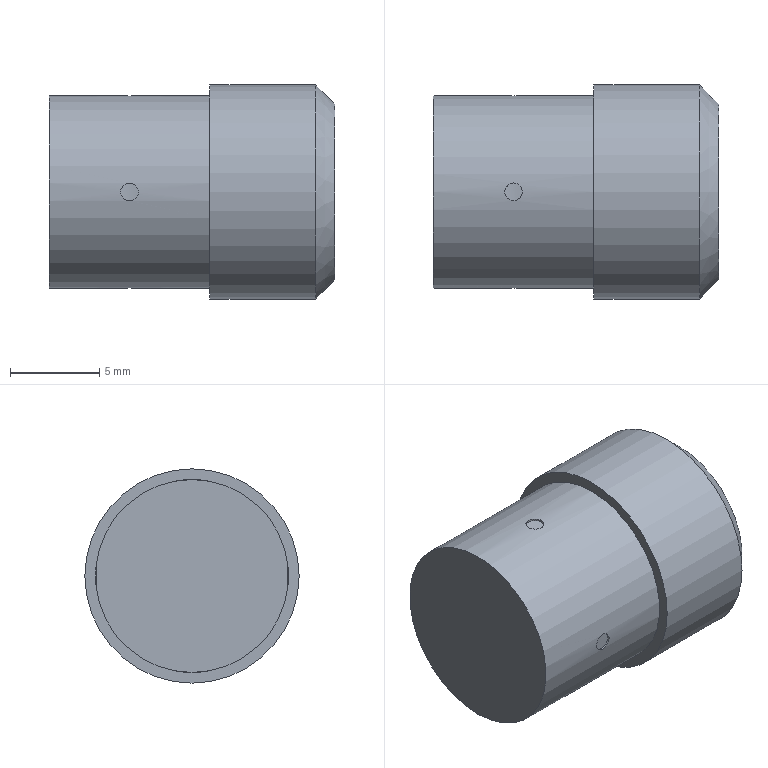Part | NX | features BREP 1 | 1 solid | 24 faces | box 16 x 12 x 12 mm | volume 1208 mm3 | cylinder 15 | plane 8 | cone 1 | commonest cylinder face diameters 1 x8 10.6 x4 9.6 x1 10.8 x1 12 x1
STEP:
#1=CARTESIAN_POINT('',(4.,0.,5.4));
#2=VERTEX_POINT('',#1);
#3=CARTESIAN_POINT('',(4.501,-0.7501,5.354));
#4=CARTESIAN_POINT('',(3.75,0.00004561,5.423));
#5=CARTESIAN_POINT('',(4.5,0.7499,5.354));
#6=CARTESIAN_POINT('',(5.25,0.0003197,5.423));
#7=CARTESIAN_POINT('',(4.501,-0.7501,5.354));
#8=CARTESIAN_POINT('',(3.75,0.00004561,5.423));
#9=CARTESIAN_POINT('',(4.5,0.7499,5.354));
#10=B_SPLINE_CURVE_WITH_KNOTS('',3,(#3,#4,#5,#6,#7,#8,#9),.UNSPECIFIED.,.T.,.F.,(1,1,1,1,1,1,1,1,1,1,1),(-0.002346,-0.001564,-0.0007819,0.,0.0007819,0.001564,0.002346,0.003128,0.00391,0.004692,0.005474),.UNSPECIFIED.);
#11=EDGE_CURVE('',#2,#2,#10,.T.);
#12=ORIENTED_EDGE('',*,*,#11,.T.);
#13=EDGE_LOOP('',(#12));
#14=FACE_BOUND('',#13,.T.);
#15=CARTESIAN_POINT('',(9.,0.,-5.4));
#16=VERTEX_POINT('',#15);
#17=CARTESIAN_POINT('',(9.,0.,0.));
#18=DIRECTION('',(-1.,0.,0.));
#19=DIRECTION('',(0.,0.,-1.));
#20=AXIS2_PLACEMENT_3D('',#17,#18,#19);
#21=CIRCLE('',#20,5.4);
#22=EDGE_CURVE('',#16,#16,#21,.T.);
#23=ORIENTED_EDGE('',*,*,#22,.T.);
#24=EDGE_LOOP('',(#23));
#25=FACE_BOUND('',#24,.T.);
#26=CARTESIAN_POINT('',(5.,0.,-5.4));
#27=VERTEX_POINT('',#26);
#28=CARTESIAN_POINT('',(4.499,-0.7501,-5.354));
#29=CARTESIAN_POINT('',(5.25,0.00004561,-5.423));
#30=CARTESIAN_POINT('',(4.5,0.7499,-5.354));
#31=CARTESIAN_POINT('',(3.75,0.0003197,-5.423));
#32=CARTESIAN_POINT('',(4.499,-0.7501,-5.354));
#33=CARTESIAN_POINT('',(5.25,0.00004561,-5.423));
#34=CARTESIAN_POINT('',(4.5,0.7499,-5.354));
#35=B_SPLINE_CURVE_WITH_KNOTS('',3,(#28,#29,#30,#31,#32,#33,#34),.UNSPECIFIED.,.T.,.F.,(1,1,1,1,1,1,1,1,1,1,1),(-0.002346,-0.001564,-0.0007819,0.,0.0007819,0.001564,0.002346,0.003128,0.00391,0.004692,0.005474),.UNSPECIFIED.);
#36=EDGE_CURVE('',#27,#27,#35,.T.);
#37=ORIENTED_EDGE('',*,*,#36,.T.);
#38=EDGE_LOOP('',(#37));
#39=FACE_BOUND('',#38,.T.);
#40=CARTESIAN_POINT('',(0.,0.,-5.4));
#41=VERTEX_POINT('',#40);
#42=CARTESIAN_POINT('',(0.,0.,0.));
#43=DIRECTION('',(1.,0.,0.));
#44=DIRECTION('',(0.,0.,-1.));
#45=AXIS2_PLACEMENT_3D('',#42,#43,#44);
#46=CIRCLE('',#45,5.4);
#47=EDGE_CURVE('',#41,#41,#46,.T.);
#48=ORIENTED_EDGE('',*,*,#47,.T.);
#49=EDGE_LOOP('',(#48));
#50=FACE_BOUND('',#49,.T.);
#51=CARTESIAN_POINT('',(4.5,5.377,0.5));
#52=VERTEX_POINT('',#51);
#53=CARTESIAN_POINT('',(5.25,5.423,-0.0007741));
#54=CARTESIAN_POINT('',(4.5,5.354,0.7501));
#55=CARTESIAN_POINT('',(3.75,5.423,0.0003559));
#56=CARTESIAN_POINT('',(4.5,5.354,-0.7499));
#57=CARTESIAN_POINT('',(5.25,5.423,-0.0007741));
#58=CARTESIAN_POINT('',(4.5,5.354,0.7501));
#59=CARTESIAN_POINT('',(3.75,5.423,0.0003559));
#60=B_SPLINE_CURVE_WITH_KNOTS('',3,(#53,#54,#55,#56,#57,#58,#59),.UNSPECIFIED.,.T.,.F.,(1,1,1,1,1,1,1,1,1,1,1),(-0.002346,-0.001564,-0.0007819,0.,0.0007819,0.001564,0.002346,0.003128,0.00391,0.004692,0.005474),.UNSPECIFIED.);
#61=EDGE_CURVE('',#52,#52,#60,.T.);
#62=ORIENTED_EDGE('',*,*,#61,.T.);
#63=EDGE_LOOP('',(#62));
#64=FACE_BOUND('',#63,.T.);
#65=CARTESIAN_POINT('',(4.5,-5.377,-0.5));
#66=VERTEX_POINT('',#65);
#67=CARTESIAN_POINT('',(5.25,-5.423,0.0007741));
#68=CARTESIAN_POINT('',(4.5,-5.354,-0.7501));
#69=CARTESIAN_POINT('',(3.75,-5.423,-0.0003559));
#70=CARTESIAN_POINT('',(4.5,-5.354,0.7499));
#71=CARTESIAN_POINT('',(5.25,-5.423,0.0007741));
#72=CARTESIAN_POINT('',(4.5,-5.354,-0.7501));
#73=CARTESIAN_POINT('',(3.75,-5.423,-0.0003559));
#74=B_SPLINE_CURVE_WITH_KNOTS('',3,(#67,#68,#69,#70,#71,#72,#73),.UNSPECIFIED.,.T.,.F.,(1,1,1,1,1,1,1,1,1,1,1),(-0.002346,-0.001564,-0.0007819,0.,0.0007819,0.001564,0.002346,0.003128,0.00391,0.004692,0.005474),.UNSPECIFIED.);
#75=EDGE_CURVE('',#66,#66,#74,.T.);
#76=ORIENTED_EDGE('',*,*,#75,.T.);
#77=EDGE_LOOP('',(#76));
#78=FACE_BOUND('',#77,.T.);
#79=CARTESIAN_POINT('',(9.,0.,0.));
#80=DIRECTION('',(1.,0.,0.));
#81=DIRECTION('',(0.,0.,1.));
#82=AXIS2_PLACEMENT_3D('',#79,#80,#81);
#83=CYLINDRICAL_SURFACE('',#82,5.4);
#84=ADVANCED_FACE('',(#14,#25,#39,#50,#64,#78),#83,.T.);
#85=ORIENTED_EDGE('',*,*,#36,.F.);
#86=EDGE_LOOP('',(#85));
#87=FACE_BOUND('',#86,.T.);
#88=CARTESIAN_POINT('',(4.,0.,-5.3));
#89=VERTEX_POINT('',#88);
#90=CARTESIAN_POINT('',(4.501,-0.7501,-5.253));
#91=CARTESIAN_POINT('',(3.75,0.00004567,-5.324));
#92=CARTESIAN_POINT('',(4.5,0.7499,-5.253));
#93=CARTESIAN_POINT('',(5.25,0.0003201,-5.324));
#94=CARTESIAN_POINT('',(4.501,-0.7501,-5.253));
#95=CARTESIAN_POINT('',(3.75,0.00004567,-5.324));
#96=CARTESIAN_POINT('',(4.5,0.7499,-5.253));
#97=B_SPLINE_CURVE_WITH_KNOTS('',3,(#90,#91,#92,#93,#94,#95,#96),.UNSPECIFIED.,.T.,.F.,(1,1,1,1,1,1,1,1,1,1,1),(-0.002346,-0.001564,-0.000782,0.,0.000782,0.001564,0.002346,0.003128,0.00391,0.004692,0.005474),.UNSPECIFIED.);
#98=EDGE_CURVE('',#89,#89,#97,.T.);
#99=ORIENTED_EDGE('',*,*,#98,.F.);
#100=EDGE_LOOP('',(#99));
#101=FACE_BOUND('',#100,.T.);
#102=CARTESIAN_POINT('',(4.5,0.,0.));
#103=DIRECTION('',(0.,0.,1.));
#104=DIRECTION('',(-1.,0.,0.));
#105=AXIS2_PLACEMENT_3D('',#102,#103,#104);
#106=CYLINDRICAL_SURFACE('',#105,0.5);
#107=ADVANCED_FACE('',(#87,#101),#106,.F.);
#108=ORIENTED_EDGE('',*,*,#22,.F.);
#109=EDGE_LOOP('',(#108));
#110=FACE_BOUND('',#109,.T.);
#111=CARTESIAN_POINT('',(9.,0.,-6.));
#112=VERTEX_POINT('',#111);
#113=CARTESIAN_POINT('',(9.,0.,0.));
#114=DIRECTION('',(1.,0.,0.));
#115=DIRECTION('',(0.,0.,-1.));
#116=AXIS2_PLACEMENT_3D('',#113,#114,#115);
#117=CIRCLE('',#116,6.);
#118=EDGE_CURVE('',#112,#112,#117,.T.);
#119=ORIENTED_EDGE('',*,*,#118,.F.);
#120=EDGE_LOOP('',(#119));
#121=FACE_BOUND('',#120,.T.);
#122=CARTESIAN_POINT('',(9.,0.,0.));
#123=DIRECTION('',(1.,0.,0.));
#124=DIRECTION('',(0.,0.,1.));
#125=AXIS2_PLACEMENT_3D('',#122,#123,#124);
#126=PLANE('',#125);
#127=ADVANCED_FACE('',(#110,#121),#126,.F.);
#128=CARTESIAN_POINT('',(5.,0.,5.3));
#129=VERTEX_POINT('',#128);
#130=CARTESIAN_POINT('',(4.499,-0.7501,5.253));
#131=CARTESIAN_POINT('',(5.25,0.00004567,5.324));
#132=CARTESIAN_POINT('',(4.5,0.7499,5.253));
#133=CARTESIAN_POINT('',(3.75,0.0003201,5.324));
#134=CARTESIAN_POINT('',(4.499,-0.7501,5.253));
#135=CARTESIAN_POINT('',(5.25,0.00004567,5.324));
#136=CARTESIAN_POINT('',(4.5,0.7499,5.253));
#137=B_SPLINE_CURVE_WITH_KNOTS('',3,(#130,#131,#132,#133,#134,#135,#136),.UNSPECIFIED.,.T.,.F.,(1,1,1,1,1,1,1,1,1,1,1),(-0.002346,-0.001564,-0.000782,0.,0.000782,0.001564,0.002346,0.003128,0.00391,0.004692,0.005474),.UNSPECIFIED.);
#138=EDGE_CURVE('',#129,#129,#137,.T.);
#139=ORIENTED_EDGE('',*,*,#138,.F.);
#140=EDGE_LOOP('',(#139));
#141=FACE_BOUND('',#140,.T.);
#142=ORIENTED_EDGE('',*,*,#11,.F.);
#143=EDGE_LOOP('',(#142));
#144=FACE_BOUND('',#143,.T.);
#145=CARTESIAN_POINT('',(4.5,0.,5.4));
#146=DIRECTION('',(0.,0.,1.));
#147=DIRECTION('',(-1.,0.,0.));
#148=AXIS2_PLACEMENT_3D('',#145,#146,#147);
#149=CYLINDRICAL_SURFACE('',#148,0.5);
#150=ADVANCED_FACE('',(#141,#144),#149,.F.);
#151=ORIENTED_EDGE('',*,*,#47,.F.);
#152=EDGE_LOOP('',(#151));
#153=FACE_BOUND('',#152,.T.);
#154=CARTESIAN_POINT('',(0.,0.,0.));
#155=DIRECTION('',(1.,0.,0.));
#156=DIRECTION('',(0.,0.,1.));
#157=AXIS2_PLACEMENT_3D('',#154,#155,#156);
#158=PLANE('',#157);
#159=ADVANCED_FACE('',(#153),#158,.F.);
#160=ORIENTED_EDGE('',*,*,#61,.F.);
#161=EDGE_LOOP('',(#160));
#162=FACE_BOUND('',#161,.T.);
#163=CARTESIAN_POINT('',(4.5,5.276,0.5));
#164=VERTEX_POINT('',#163);
#165=CARTESIAN_POINT('',(3.75,5.324,-0.0007718));
#166=CARTESIAN_POINT('',(4.5,5.253,0.7501));
#167=CARTESIAN_POINT('',(5.25,5.324,0.0003567));
#168=CARTESIAN_POINT('',(4.5,5.253,-0.7499));
#169=CARTESIAN_POINT('',(3.75,5.324,-0.0007718));
#170=CARTESIAN_POINT('',(4.5,5.253,0.7501));
#171=CARTESIAN_POINT('',(5.25,5.324,0.0003567));
#172=B_SPLINE_CURVE_WITH_KNOTS('',3,(#165,#166,#167,#168,#169,#170,#171),.UNSPECIFIED.,.T.,.F.,(1,1,1,1,1,1,1,1,1,1,1),(-0.002346,-0.001564,-0.000782,0.,0.000782,0.001564,0.002346,0.003128,0.00391,0.004692,0.005474),.UNSPECIFIED.);
#173=EDGE_CURVE('',#164,#164,#172,.T.);
#174=ORIENTED_EDGE('',*,*,#173,.F.);
#175=EDGE_LOOP('',(#174));
#176=FACE_BOUND('',#175,.T.);
#177=CARTESIAN_POINT('',(4.5,0.,0.));
#178=DIRECTION('',(0.,-1.,0.));
#179=DIRECTION('',(0.,0.,1.));
#180=AXIS2_PLACEMENT_3D('',#177,#178,#179);
#181=CYLINDRICAL_SURFACE('',#180,0.5);
#182=ADVANCED_FACE('',(#162,#176),#181,.F.);
#183=ORIENTED_EDGE('',*,*,#75,.F.);
#184=EDGE_LOOP('',(#183));
#185=FACE_BOUND('',#184,.T.);
#186=CARTESIAN_POINT('',(4.5,-5.276,0.5));
#187=VERTEX_POINT('',#186);
#188=CARTESIAN_POINT('',(5.25,-5.324,-0.0007718));
#189=CARTESIAN_POINT('',(4.5,-5.253,0.7501));
#190=CARTESIAN_POINT('',(3.75,-5.324,0.0003567));
#191=CARTESIAN_POINT('',(4.5,-5.253,-0.7499));
#192=CARTESIAN_POINT('',(5.25,-5.324,-0.0007718));
#193=CARTESIAN_POINT('',(4.5,-5.253,0.7501));
#194=CARTESIAN_POINT('',(3.75,-5.324,0.0003567));
#195=B_SPLINE_CURVE_WITH_KNOTS('',3,(#188,#189,#190,#191,#192,#193,#194),.UNSPECIFIED.,.T.,.F.,(1,1,1,1,1,1,1,1,1,1,1),(-0.002346,-0.001564,-0.000782,0.,0.000782,0.001564,0.002346,0.003128,0.00391,0.004692,0.005474),.UNSPECIFIED.);
#196=EDGE_CURVE('',#187,#187,#195,.T.);
#197=ORIENTED_EDGE('',*,*,#196,.F.);
#198=EDGE_LOOP('',(#197));
#199=FACE_BOUND('',#198,.T.);
#200=CARTESIAN_POINT('',(4.5,0.,0.));
#201=DIRECTION('',(0.,-1.,0.));
#202=DIRECTION('',(0.,0.,1.));
#203=AXIS2_PLACEMENT_3D('',#200,#201,#202);
#204=CYLINDRICAL_SURFACE('',#203,0.5);
#205=ADVANCED_FACE('',(#185,#199),#204,.F.);
#206=ORIENTED_EDGE('',*,*,#98,.T.);
#207=EDGE_LOOP('',(#206));
#208=FACE_BOUND('',#207,.T.);
#209=CARTESIAN_POINT('',(9.,0.,0.));
#210=DIRECTION('',(1.,0.,0.));
#211=DIRECTION('',(0.,0.,1.));
#212=AXIS2_PLACEMENT_3D('',#209,#210,#211);
#213=CYLINDRICAL_SURFACE('',#212,5.3);
#214=ADVANCED_FACE('',(#208),#213,.T.);
#215=CARTESIAN_POINT('',(14.927,0.,-6.));
#216=VERTEX_POINT('',#215);
#217=CARTESIAN_POINT('',(14.927,0.,0.));
#218=DIRECTION('',(-1.,0.,0.));
#219=DIRECTION('',(0.,0.,-1.));
#220=AXIS2_PLACEMENT_3D('',#217,#218,#219);
#221=CIRCLE('',#220,6.);
#222=EDGE_CURVE('',#216,#216,#221,.T.);
#223=ORIENTED_EDGE('',*,*,#222,.T.);
#224=EDGE_LOOP('',(#223));
#225=FACE_BOUND('',#224,.T.);
#226=ORIENTED_EDGE('',*,*,#118,.T.);
#227=EDGE_LOOP('',(#226));
#228=FACE_BOUND('',#227,.T.);
#229=CARTESIAN_POINT('',(16.,0.,0.));
#230=DIRECTION('',(1.,0.,0.));
#231=DIRECTION('',(0.,0.,1.));
#232=AXIS2_PLACEMENT_3D('',#229,#230,#231);
#233=CYLINDRICAL_SURFACE('',#232,6.);
#234=ADVANCED_FACE('',(#225,#228),#233,.T.);
#235=ORIENTED_EDGE('',*,*,#138,.T.);
#236=EDGE_LOOP('',(#235));
#237=FACE_BOUND('',#236,.T.);
#238=CARTESIAN_POINT('',(9.,0.,0.));
#239=DIRECTION('',(1.,0.,0.));
#240=DIRECTION('',(0.,0.,1.));
#241=AXIS2_PLACEMENT_3D('',#238,#239,#240);
#242=CYLINDRICAL_SURFACE('',#241,5.3);
#243=ADVANCED_FACE('',(#237),#242,.T.);
#244=ORIENTED_EDGE('',*,*,#173,.T.);
#245=EDGE_LOOP('',(#244));
#246=FACE_BOUND('',#245,.T.);
#247=CARTESIAN_POINT('',(9.,0.,0.));
#248=DIRECTION('',(1.,0.,0.));
#249=DIRECTION('',(0.,0.,1.));
#250=AXIS2_PLACEMENT_3D('',#247,#248,#249);
#251=CYLINDRICAL_SURFACE('',#250,5.3);
#252=ADVANCED_FACE('',(#246),#251,.T.);
#253=ORIENTED_EDGE('',*,*,#196,.T.);
#254=EDGE_LOOP('',(#253));
#255=FACE_BOUND('',#254,.T.);
#256=CARTESIAN_POINT('',(9.,0.,0.));
#257=DIRECTION('',(1.,0.,0.));
#258=DIRECTION('',(0.,0.,1.));
#259=AXIS2_PLACEMENT_3D('',#256,#257,#258);
#260=CYLINDRICAL_SURFACE('',#259,5.3);
#261=ADVANCED_FACE('',(#255),#260,.T.);
#262=ORIENTED_EDGE('',*,*,#222,.F.);
#263=EDGE_LOOP('',(#262));
#264=FACE_BOUND('',#263,.T.);
#265=CARTESIAN_POINT('',(16.,0.,4.927));
#266=VERTEX_POINT('',#265);
#267=CARTESIAN_POINT('',(16.,0.,0.));
#268=DIRECTION('',(-1.,0.,0.));
#269=DIRECTION('',(0.,0.,1.));
#270=AXIS2_PLACEMENT_3D('',#267,#268,#269);
#271=CIRCLE('',#270,4.927);
#272=EDGE_CURVE('',#266,#266,#271,.T.);
#273=ORIENTED_EDGE('',*,*,#272,.T.);
#274=EDGE_LOOP('',(#273));
#275=FACE_BOUND('',#274,.T.);
#276=CARTESIAN_POINT('',(14.927,0.,0.));
#277=DIRECTION('',(-1.,0.,0.));
#278=DIRECTION('',(0.,0.,-1.));
#279=AXIS2_PLACEMENT_3D('',#276,#277,#278);
#280=CONICAL_SURFACE('',#279,6.,0.7854);
#281=ADVANCED_FACE('',(#264,#275),#280,.T.);
#282=ORIENTED_EDGE('',*,*,#272,.F.);
#283=EDGE_LOOP('',(#282));
#284=FACE_BOUND('',#283,.T.);
#285=CARTESIAN_POINT('',(16.,0.,-4.8));
#286=VERTEX_POINT('',#285);
#287=CARTESIAN_POINT('',(16.,0.,0.));
#288=DIRECTION('',(1.,0.,0.));
#289=DIRECTION('',(0.,0.,-1.));
#290=AXIS2_PLACEMENT_3D('',#287,#288,#289);
#291=CIRCLE('',#290,4.8);
#292=EDGE_CURVE('',#286,#286,#291,.T.);
#293=ORIENTED_EDGE('',*,*,#292,.F.);
#294=EDGE_LOOP('',(#293));
#295=FACE_BOUND('',#294,.T.);
#296=CARTESIAN_POINT('',(16.,4.926,0.));
#297=DIRECTION('',(-1.,0.,0.));
#298=DIRECTION('',(0.,0.,-1.));
#299=AXIS2_PLACEMENT_3D('',#296,#297,#298);
#300=PLANE('',#299);
#301=ADVANCED_FACE('',(#284,#295),#300,.F.);
#302=CARTESIAN_POINT('',(10.4,0.,-4.8));
#303=VERTEX_POINT('',#302);
#304=CARTESIAN_POINT('',(10.4,0.,0.));
#305=DIRECTION('',(1.,0.,0.));
#306=DIRECTION('',(0.,0.,-1.));
#307=AXIS2_PLACEMENT_3D('',#304,#305,#306);
#308=CIRCLE('',#307,4.8);
#309=EDGE_CURVE('',#303,#303,#308,.T.);
#310=ORIENTED_EDGE('',*,*,#309,.F.);
#311=EDGE_LOOP('',(#310));
#312=FACE_BOUND('',#311,.T.);
#313=ORIENTED_EDGE('',*,*,#292,.T.);
#314=EDGE_LOOP('',(#313));
#315=FACE_BOUND('',#314,.T.);
#316=CARTESIAN_POINT('',(10.4,0.,0.));
#317=DIRECTION('',(1.,0.,0.));
#318=DIRECTION('',(0.,0.,1.));
#319=AXIS2_PLACEMENT_3D('',#316,#317,#318);
#320=CYLINDRICAL_SURFACE('',#319,4.8);
#321=ADVANCED_FACE('',(#312,#315),#320,.F.);
#322=ORIENTED_EDGE('',*,*,#309,.T.);
#323=EDGE_LOOP('',(#322));
#324=FACE_BOUND('',#323,.T.);
#325=CARTESIAN_POINT('',(10.4,0.,-2.9));
#326=VERTEX_POINT('',#325);
#327=CARTESIAN_POINT('',(10.4,0.,-2.4));
#328=DIRECTION('',(-1.,0.,0.));
#329=DIRECTION('',(0.,0.,-1.));
#330=AXIS2_PLACEMENT_3D('',#327,#328,#329);
#331=CIRCLE('',#330,0.5);
#332=EDGE_CURVE('',#326,#326,#331,.T.);
#333=ORIENTED_EDGE('',*,*,#332,.T.);
#334=EDGE_LOOP('',(#333));
#335=FACE_BOUND('',#334,.T.);
#336=CARTESIAN_POINT('',(10.4,2.4,-0.5));
#337=VERTEX_POINT('',#336);
#338=CARTESIAN_POINT('',(10.4,2.4,0.));
#339=DIRECTION('',(-1.,0.,0.));
#340=DIRECTION('',(0.,0.,-1.));
#341=AXIS2_PLACEMENT_3D('',#338,#339,#340);
#342=CIRCLE('',#341,0.5);
#343=EDGE_CURVE('',#337,#337,#342,.T.);
#344=ORIENTED_EDGE('',*,*,#343,.T.);
#345=EDGE_LOOP('',(#344));
#346=FACE_BOUND('',#345,.T.);
#347=CARTESIAN_POINT('',(10.4,-2.4,-0.5));
#348=VERTEX_POINT('',#347);
#349=CARTESIAN_POINT('',(10.4,-2.4,0.));
#350=DIRECTION('',(-1.,0.,0.));
#351=DIRECTION('',(0.,0.,-1.));
#352=AXIS2_PLACEMENT_3D('',#349,#350,#351);
#353=CIRCLE('',#352,0.5);
#354=EDGE_CURVE('',#348,#348,#353,.T.);
#355=ORIENTED_EDGE('',*,*,#354,.T.);
#356=EDGE_LOOP('',(#355));
#357=FACE_BOUND('',#356,.T.);
#358=CARTESIAN_POINT('',(10.4,0.,1.9));
#359=VERTEX_POINT('',#358);
#360=CARTESIAN_POINT('',(10.4,0.,2.4));
#361=DIRECTION('',(-1.,0.,0.));
#362=DIRECTION('',(0.,0.,-1.));
#363=AXIS2_PLACEMENT_3D('',#360,#361,#362);
#364=CIRCLE('',#363,0.5);
#365=EDGE_CURVE('',#359,#359,#364,.T.);
#366=ORIENTED_EDGE('',*,*,#365,.T.);
#367=EDGE_LOOP('',(#366));
#368=FACE_BOUND('',#367,.T.);
#369=CARTESIAN_POINT('',(10.4,0.,0.));
#370=DIRECTION('',(1.,0.,0.));
#371=DIRECTION('',(0.,0.,1.));
#372=AXIS2_PLACEMENT_3D('',#369,#370,#371);
#373=PLANE('',#372);
#374=ADVANCED_FACE('',(#324,#335,#346,#357,#368),#373,.T.);
#375=ORIENTED_EDGE('',*,*,#332,.F.);
#376=EDGE_LOOP('',(#375));
#377=FACE_BOUND('',#376,.T.);
#378=CARTESIAN_POINT('',(16.,0.,-2.9));
#379=VERTEX_POINT('',#378);
#380=CARTESIAN_POINT('',(16.,0.,-2.4));
#381=DIRECTION('',(-1.,0.,0.));
#382=DIRECTION('',(0.,0.,-1.));
#383=AXIS2_PLACEMENT_3D('',#380,#381,#382);
#384=CIRCLE('',#383,0.5);
#385=EDGE_CURVE('',#379,#379,#384,.T.);
#386=ORIENTED_EDGE('',*,*,#385,.T.);
#387=EDGE_LOOP('',(#386));
#388=FACE_BOUND('',#387,.T.);
#389=CARTESIAN_POINT('',(10.4,0.,-2.4));
#390=DIRECTION('',(1.,0.,0.));
#391=DIRECTION('',(0.,0.,1.));
#392=AXIS2_PLACEMENT_3D('',#389,#390,#391);
#393=CYLINDRICAL_SURFACE('',#392,0.5);
#394=ADVANCED_FACE('',(#377,#388),#393,.T.);
#395=ORIENTED_EDGE('',*,*,#343,.F.);
#396=EDGE_LOOP('',(#395));
#397=FACE_BOUND('',#396,.T.);
#398=CARTESIAN_POINT('',(16.,2.4,-0.5));
#399=VERTEX_POINT('',#398);
#400=CARTESIAN_POINT('',(16.,2.4,0.));
#401=DIRECTION('',(-1.,0.,0.));
#402=DIRECTION('',(0.,0.,-1.));
#403=AXIS2_PLACEMENT_3D('',#400,#401,#402);
#404=CIRCLE('',#403,0.5);
#405=EDGE_CURVE('',#399,#399,#404,.T.);
#406=ORIENTED_EDGE('',*,*,#405,.T.);
#407=EDGE_LOOP('',(#406));
#408=FACE_BOUND('',#407,.T.);
#409=CARTESIAN_POINT('',(10.4,2.4,0.));
#410=DIRECTION('',(1.,0.,0.));
#411=DIRECTION('',(0.,0.,1.));
#412=AXIS2_PLACEMENT_3D('',#409,#410,#411);
#413=CYLINDRICAL_SURFACE('',#412,0.5);
#414=ADVANCED_FACE('',(#397,#408),#413,.T.);
#415=ORIENTED_EDGE('',*,*,#354,.F.);
#416=EDGE_LOOP('',(#415));
#417=FACE_BOUND('',#416,.T.);
#418=CARTESIAN_POINT('',(16.,-2.4,-0.5));
#419=VERTEX_POINT('',#418);
#420=CARTESIAN_POINT('',(16.,-2.4,0.));
#421=DIRECTION('',(-1.,0.,0.));
#422=DIRECTION('',(0.,0.,-1.));
#423=AXIS2_PLACEMENT_3D('',#420,#421,#422);
#424=CIRCLE('',#423,0.5);
#425=EDGE_CURVE('',#419,#419,#424,.T.);
#426=ORIENTED_EDGE('',*,*,#425,.T.);
#427=EDGE_LOOP('',(#426));
#428=FACE_BOUND('',#427,.T.);
#429=CARTESIAN_POINT('',(10.4,-2.4,0.));
#430=DIRECTION('',(1.,0.,0.));
#431=DIRECTION('',(0.,0.,1.));
#432=AXIS2_PLACEMENT_3D('',#429,#430,#431);
#433=CYLINDRICAL_SURFACE('',#432,0.5);
#434=ADVANCED_FACE('',(#417,#428),#433,.T.);
#435=ORIENTED_EDGE('',*,*,#365,.F.);
#436=EDGE_LOOP('',(#435));
#437=FACE_BOUND('',#436,.T.);
#438=CARTESIAN_POINT('',(16.,0.,1.9));
#439=VERTEX_POINT('',#438);
#440=CARTESIAN_POINT('',(16.,0.,2.4));
#441=DIRECTION('',(-1.,0.,0.));
#442=DIRECTION('',(0.,0.,-1.));
#443=AXIS2_PLACEMENT_3D('',#440,#441,#442);
#444=CIRCLE('',#443,0.5);
#445=EDGE_CURVE('',#439,#439,#444,.T.);
#446=ORIENTED_EDGE('',*,*,#445,.T.);
#447=EDGE_LOOP('',(#446));
#448=FACE_BOUND('',#447,.T.);
#449=CARTESIAN_POINT('',(10.4,0.,2.4));
#450=DIRECTION('',(1.,0.,0.));
#451=DIRECTION('',(0.,0.,1.));
#452=AXIS2_PLACEMENT_3D('',#449,#450,#451);
#453=CYLINDRICAL_SURFACE('',#452,0.5);
#454=ADVANCED_FACE('',(#437,#448),#453,.T.);
#455=ORIENTED_EDGE('',*,*,#385,.F.);
#456=EDGE_LOOP('',(#455));
#457=FACE_BOUND('',#456,.T.);
#458=CARTESIAN_POINT('',(16.,4.926,0.));
#459=DIRECTION('',(-1.,0.,0.));
#460=DIRECTION('',(0.,0.,-1.));
#461=AXIS2_PLACEMENT_3D('',#458,#459,#460);
#462=PLANE('',#461);
#463=ADVANCED_FACE('',(#457),#462,.F.);
#464=ORIENTED_EDGE('',*,*,#405,.F.);
#465=EDGE_LOOP('',(#464));
#466=FACE_BOUND('',#465,.T.);
#467=CARTESIAN_POINT('',(16.,4.926,0.));
#468=DIRECTION('',(-1.,0.,0.));
#469=DIRECTION('',(0.,0.,-1.));
#470=AXIS2_PLACEMENT_3D('',#467,#468,#469);
#471=PLANE('',#470);
#472=ADVANCED_FACE('',(#466),#471,.F.);
#473=ORIENTED_EDGE('',*,*,#425,.F.);
#474=EDGE_LOOP('',(#473));
#475=FACE_BOUND('',#474,.T.);
#476=CARTESIAN_POINT('',(16.,4.926,0.));
#477=DIRECTION('',(-1.,0.,0.));
#478=DIRECTION('',(0.,0.,-1.));
#479=AXIS2_PLACEMENT_3D('',#476,#477,#478);
#480=PLANE('',#479);
#481=ADVANCED_FACE('',(#475),#480,.F.);
#482=ORIENTED_EDGE('',*,*,#445,.F.);
#483=EDGE_LOOP('',(#482));
#484=FACE_BOUND('',#483,.T.);
#485=CARTESIAN_POINT('',(16.,4.926,0.));
#486=DIRECTION('',(-1.,0.,0.));
#487=DIRECTION('',(0.,0.,-1.));
#488=AXIS2_PLACEMENT_3D('',#485,#486,#487);
#489=PLANE('',#488);
#490=ADVANCED_FACE('',(#484),#489,.F.);
#491=CLOSED_SHELL('',(#84,#107,#127,#150,#159,#182,#205,#214,#234,#243,#252,#261,#281,#301,#321,#374,#394,#414,#434,#454,#463,#472,#481,#490));
#492=MANIFOLD_SOLID_BREP('',#491);
#493=(LENGTH_UNIT()NAMED_UNIT(*)SI_UNIT(.MILLI.,.METRE.));
#494=UNCERTAINTY_MEASURE_WITH_UNIT(LENGTH_MEASURE(0.0508),#493,'','');
#495=(NAMED_UNIT(*)PLANE_ANGLE_UNIT()SI_UNIT($,.RADIAN.));
#496=(NAMED_UNIT(*)SI_UNIT($,.STERADIAN.)SOLID_ANGLE_UNIT());
#497=(GEOMETRIC_REPRESENTATION_CONTEXT(3)GLOBAL_UNCERTAINTY_ASSIGNED_CONTEXT((#494))GLOBAL_UNIT_ASSIGNED_CONTEXT((#493,#495,#496))REPRESENTATION_CONTEXT('',''));
#498=ADVANCED_BREP_SHAPE_REPRESENTATION('',(#492),#497);